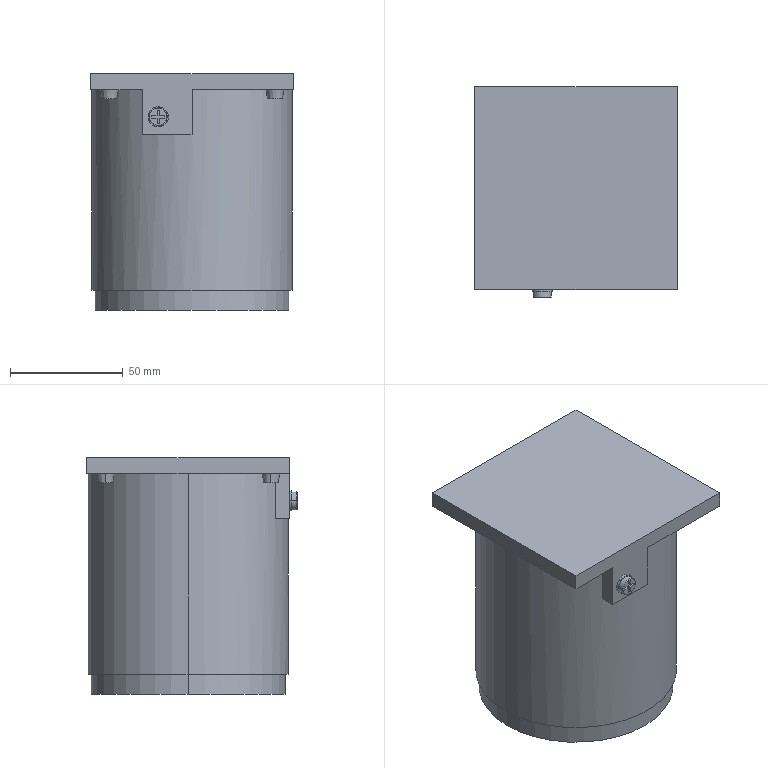Part | STEP file | 0229_Z_5IK40AW-GAL20J_2 | 1 solid | 48 faces | box 90 x 93.5 x 105 mm | volume 664924 mm3 | plane 30 | cylinder 8 | cone 8 | torus 2 | commonest cylinder face diameters 8 x2 9 x2 86 x2 89 x2